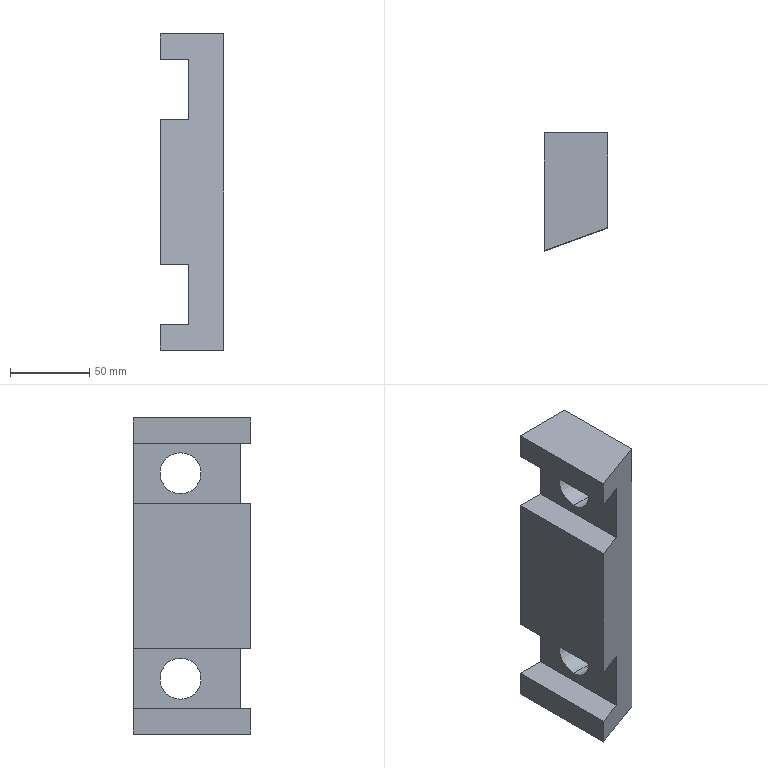Part | SolidWorks | features ICE 2, Extrusion 1, MirrorPattern 1 | 1 solid | 18 faces | box 40 x 74.559 x 200 mm | volume 417359 mm3 | plane 14 | cylinder 4 | commonest cylinder face diameters 26 x4
STEP:
#1=CARTESIAN_POINT('',(40.,44.559,78.));
#2=VERTEX_POINT('',#1);
#3=CARTESIAN_POINT('',(40.,44.559,52.));
#4=VERTEX_POINT('',#3);
#5=CARTESIAN_POINT('',(40.,44.559,65.));
#6=DIRECTION('',(1.,0.,0.));
#7=DIRECTION('',(0.,-1.,0.));
#8=AXIS2_PLACEMENT_3D('',#5,#6,#7);
#9=CIRCLE('',#8,13.);
#10=EDGE_CURVE('',#2,#4,#9,.T.);
#11=ORIENTED_EDGE('',*,*,#10,.T.);
#12=CARTESIAN_POINT('',(18.,44.559,52.));
#13=VERTEX_POINT('',#12);
#14=CARTESIAN_POINT('',(60.,44.559,52.));
#15=DIRECTION('',(-1.,0.,0.));
#16=VECTOR('',#15,1000.);
#17=LINE('',#14,#16);
#18=EDGE_CURVE('',#4,#13,#17,.T.);
#19=ORIENTED_EDGE('',*,*,#18,.T.);
#20=CARTESIAN_POINT('',(18.,44.559,78.));
#21=VERTEX_POINT('',#20);
#22=CARTESIAN_POINT('',(18.,44.559,65.));
#23=DIRECTION('',(1.,0.,0.));
#24=DIRECTION('',(0.,0.,1.));
#25=AXIS2_PLACEMENT_3D('',#22,#23,#24);
#26=CIRCLE('',#25,13.);
#27=EDGE_CURVE('',#21,#13,#26,.T.);
#28=ORIENTED_EDGE('',*,*,#27,.F.);
#29=CARTESIAN_POINT('',(60.,44.559,78.));
#30=DIRECTION('',(-1.,0.,0.));
#31=VECTOR('',#30,1000.);
#32=LINE('',#29,#31);
#33=EDGE_CURVE('',#2,#21,#32,.T.);
#34=ORIENTED_EDGE('',*,*,#33,.F.);
#35=EDGE_LOOP('',(#11,#19,#28,#34));
#36=FACE_OUTER_BOUND('',#35,.T.);
#37=CARTESIAN_POINT('',(60.,44.559,65.));
#38=DIRECTION('',(-1.,0.,0.));
#39=DIRECTION('',(0.,0.,1.));
#40=AXIS2_PLACEMENT_3D('',#37,#38,#39);
#41=CYLINDRICAL_SURFACE('',#40,13.);
#42=ADVANCED_FACE('',(#36),#41,.F.);
#43=CARTESIAN_POINT('',(40.,44.559,-52.));
#44=VERTEX_POINT('',#43);
#45=CARTESIAN_POINT('',(40.,44.559,-78.));
#46=VERTEX_POINT('',#45);
#47=CARTESIAN_POINT('',(40.,44.559,-65.));
#48=DIRECTION('',(1.,0.,0.));
#49=DIRECTION('',(0.,-1.,0.));
#50=AXIS2_PLACEMENT_3D('',#47,#48,#49);
#51=CIRCLE('',#50,13.);
#52=EDGE_CURVE('',#44,#46,#51,.T.);
#53=ORIENTED_EDGE('',*,*,#52,.T.);
#54=CARTESIAN_POINT('',(18.,44.559,-78.));
#55=VERTEX_POINT('',#54);
#56=CARTESIAN_POINT('',(60.,44.559,-78.));
#57=DIRECTION('',(-1.,0.,0.));
#58=VECTOR('',#57,1000.);
#59=LINE('',#56,#58);
#60=EDGE_CURVE('',#46,#55,#59,.T.);
#61=ORIENTED_EDGE('',*,*,#60,.T.);
#62=CARTESIAN_POINT('',(18.,44.559,-52.));
#63=VERTEX_POINT('',#62);
#64=CARTESIAN_POINT('',(18.,44.559,-65.));
#65=DIRECTION('',(1.,0.,0.));
#66=DIRECTION('',(0.,0.,1.));
#67=AXIS2_PLACEMENT_3D('',#64,#65,#66);
#68=CIRCLE('',#67,13.);
#69=EDGE_CURVE('',#63,#55,#68,.T.);
#70=ORIENTED_EDGE('',*,*,#69,.F.);
#71=CARTESIAN_POINT('',(60.,44.559,-52.));
#72=DIRECTION('',(-1.,0.,0.));
#73=VECTOR('',#72,1000.);
#74=LINE('',#71,#73);
#75=EDGE_CURVE('',#44,#63,#74,.T.);
#76=ORIENTED_EDGE('',*,*,#75,.F.);
#77=EDGE_LOOP('',(#53,#61,#70,#76));
#78=FACE_OUTER_BOUND('',#77,.T.);
#79=CARTESIAN_POINT('',(60.,44.559,-65.));
#80=DIRECTION('',(-1.,0.,0.));
#81=DIRECTION('',(0.,0.,1.));
#82=AXIS2_PLACEMENT_3D('',#79,#80,#81);
#83=CYLINDRICAL_SURFACE('',#82,13.);
#84=ADVANCED_FACE('',(#78),#83,.F.);
#85=CARTESIAN_POINT('',(18.,6.551,84.));
#86=VERTEX_POINT('',#85);
#87=CARTESIAN_POINT('',(0.,0.,84.));
#88=VERTEX_POINT('',#87);
#89=CARTESIAN_POINT('',(40.,14.559,84.));
#90=DIRECTION('',(-0.9397,-0.342,0.));
#91=VECTOR('',#90,1000.);
#92=LINE('',#89,#91);
#93=EDGE_CURVE('',#86,#88,#92,.T.);
#94=ORIENTED_EDGE('',*,*,#93,.F.);
#95=CARTESIAN_POINT('',(18.,6.551,46.));
#96=VERTEX_POINT('',#95);
#97=CARTESIAN_POINT('',(18.,6.551,100.));
#98=DIRECTION('',(0.,0.,1.));
#99=VECTOR('',#98,1000.);
#100=LINE('',#97,#99);
#101=EDGE_CURVE('',#96,#86,#100,.T.);
#102=ORIENTED_EDGE('',*,*,#101,.F.);
#103=CARTESIAN_POINT('',(0.,0.,46.));
#104=VERTEX_POINT('',#103);
#105=CARTESIAN_POINT('',(40.,14.559,46.));
#106=DIRECTION('',(0.9397,0.342,0.));
#107=VECTOR('',#106,1000.);
#108=LINE('',#105,#107);
#109=EDGE_CURVE('',#104,#96,#108,.T.);
#110=ORIENTED_EDGE('',*,*,#109,.F.);
#111=CARTESIAN_POINT('',(0.,0.,-46.));
#112=VERTEX_POINT('',#111);
#113=CARTESIAN_POINT('',(0.,0.,100.));
#114=DIRECTION('',(0.,0.,-1.));
#115=VECTOR('',#114,1000.);
#116=LINE('',#113,#115);
#117=EDGE_CURVE('',#104,#112,#116,.T.);
#118=ORIENTED_EDGE('',*,*,#117,.T.);
#119=CARTESIAN_POINT('',(18.,6.551,-46.));
#120=VERTEX_POINT('',#119);
#121=CARTESIAN_POINT('',(40.,14.559,-46.));
#122=DIRECTION('',(0.9397,0.342,0.));
#123=VECTOR('',#122,1000.);
#124=LINE('',#121,#123);
#125=EDGE_CURVE('',#112,#120,#124,.T.);
#126=ORIENTED_EDGE('',*,*,#125,.T.);
#127=CARTESIAN_POINT('',(18.,6.551,-84.));
#128=VERTEX_POINT('',#127);
#129=CARTESIAN_POINT('',(18.,6.551,100.));
#130=DIRECTION('',(0.,0.,1.));
#131=VECTOR('',#130,1000.);
#132=LINE('',#129,#131);
#133=EDGE_CURVE('',#128,#120,#132,.T.);
#134=ORIENTED_EDGE('',*,*,#133,.F.);
#135=CARTESIAN_POINT('',(0.,0.,-84.));
#136=VERTEX_POINT('',#135);
#137=CARTESIAN_POINT('',(40.,14.559,-84.));
#138=DIRECTION('',(-0.9397,-0.342,0.));
#139=VECTOR('',#138,1000.);
#140=LINE('',#137,#139);
#141=EDGE_CURVE('',#128,#136,#140,.T.);
#142=ORIENTED_EDGE('',*,*,#141,.T.);
#143=CARTESIAN_POINT('',(0.,0.,-100.));
#144=VERTEX_POINT('',#143);
#145=CARTESIAN_POINT('',(0.,0.,100.));
#146=DIRECTION('',(0.,0.,-1.));
#147=VECTOR('',#146,1000.);
#148=LINE('',#145,#147);
#149=EDGE_CURVE('',#136,#144,#148,.T.);
#150=ORIENTED_EDGE('',*,*,#149,.T.);
#151=CARTESIAN_POINT('',(40.,14.559,-100.));
#152=VERTEX_POINT('',#151);
#153=CARTESIAN_POINT('',(40.,14.559,-100.));
#154=DIRECTION('',(0.9397,0.342,0.));
#155=VECTOR('',#154,1000.);
#156=LINE('',#153,#155);
#157=EDGE_CURVE('',#144,#152,#156,.T.);
#158=ORIENTED_EDGE('',*,*,#157,.T.);
#159=CARTESIAN_POINT('',(40.,14.559,100.));
#160=VERTEX_POINT('',#159);
#161=CARTESIAN_POINT('',(40.,14.559,100.));
#162=DIRECTION('',(0.,0.,-1.));
#163=VECTOR('',#162,1000.);
#164=LINE('',#161,#163);
#165=EDGE_CURVE('',#160,#152,#164,.T.);
#166=ORIENTED_EDGE('',*,*,#165,.F.);
#167=CARTESIAN_POINT('',(0.,0.,100.));
#168=VERTEX_POINT('',#167);
#169=CARTESIAN_POINT('',(40.,14.559,100.));
#170=DIRECTION('',(0.9397,0.342,0.));
#171=VECTOR('',#170,1000.);
#172=LINE('',#169,#171);
#173=EDGE_CURVE('',#168,#160,#172,.T.);
#174=ORIENTED_EDGE('',*,*,#173,.F.);
#175=CARTESIAN_POINT('',(0.,0.,100.));
#176=DIRECTION('',(0.,0.,-1.));
#177=VECTOR('',#176,1000.);
#178=LINE('',#175,#177);
#179=EDGE_CURVE('',#168,#88,#178,.T.);
#180=ORIENTED_EDGE('',*,*,#179,.T.);
#181=EDGE_LOOP('',(#94,#102,#110,#118,#126,#134,#142,#150,#158,#166,#174,#180));
#182=FACE_OUTER_BOUND('',#181,.T.);
#183=CARTESIAN_POINT('',(40.,14.559,100.));
#184=DIRECTION('',(-0.342,0.9397,0.));
#185=DIRECTION('',(-0.9397,-0.342,0.));
#186=AXIS2_PLACEMENT_3D('',#183,#184,#185);
#187=PLANE('',#186);
#188=ADVANCED_FACE('',(#182),#187,.F.);
#189=CARTESIAN_POINT('',(0.,74.559,84.));
#190=VERTEX_POINT('',#189);
#191=CARTESIAN_POINT('',(18.,74.559,84.));
#192=VERTEX_POINT('',#191);
#193=CARTESIAN_POINT('',(0.,74.559,84.));
#194=DIRECTION('',(1.,0.,0.));
#195=VECTOR('',#194,1000.);
#196=LINE('',#193,#195);
#197=EDGE_CURVE('',#190,#192,#196,.T.);
#198=ORIENTED_EDGE('',*,*,#197,.F.);
#199=CARTESIAN_POINT('',(0.,74.559,100.));
#200=VERTEX_POINT('',#199);
#201=CARTESIAN_POINT('',(0.,74.559,100.));
#202=DIRECTION('',(0.,0.,-1.));
#203=VECTOR('',#202,1000.);
#204=LINE('',#201,#203);
#205=EDGE_CURVE('',#200,#190,#204,.T.);
#206=ORIENTED_EDGE('',*,*,#205,.F.);
#207=CARTESIAN_POINT('',(40.,74.559,100.));
#208=VERTEX_POINT('',#207);
#209=CARTESIAN_POINT('',(0.,74.559,100.));
#210=DIRECTION('',(-1.,0.,0.));
#211=VECTOR('',#210,1000.);
#212=LINE('',#209,#211);
#213=EDGE_CURVE('',#208,#200,#212,.T.);
#214=ORIENTED_EDGE('',*,*,#213,.F.);
#215=CARTESIAN_POINT('',(40.,74.559,-100.));
#216=VERTEX_POINT('',#215);
#217=CARTESIAN_POINT('',(40.,74.559,100.));
#218=DIRECTION('',(0.,0.,-1.));
#219=VECTOR('',#218,1000.);
#220=LINE('',#217,#219);
#221=EDGE_CURVE('',#208,#216,#220,.T.);
#222=ORIENTED_EDGE('',*,*,#221,.T.);
#223=CARTESIAN_POINT('',(0.,74.559,-100.));
#224=VERTEX_POINT('',#223);
#225=CARTESIAN_POINT('',(0.,74.559,-100.));
#226=DIRECTION('',(-1.,0.,0.));
#227=VECTOR('',#226,1000.);
#228=LINE('',#225,#227);
#229=EDGE_CURVE('',#216,#224,#228,.T.);
#230=ORIENTED_EDGE('',*,*,#229,.T.);
#231=CARTESIAN_POINT('',(0.,74.559,-84.));
#232=VERTEX_POINT('',#231);
#233=CARTESIAN_POINT('',(0.,74.559,100.));
#234=DIRECTION('',(0.,0.,-1.));
#235=VECTOR('',#234,1000.);
#236=LINE('',#233,#235);
#237=EDGE_CURVE('',#232,#224,#236,.T.);
#238=ORIENTED_EDGE('',*,*,#237,.F.);
#239=CARTESIAN_POINT('',(18.,74.559,-84.));
#240=VERTEX_POINT('',#239);
#241=CARTESIAN_POINT('',(0.,74.559,-84.));
#242=DIRECTION('',(1.,0.,0.));
#243=VECTOR('',#242,1000.);
#244=LINE('',#241,#243);
#245=EDGE_CURVE('',#232,#240,#244,.T.);
#246=ORIENTED_EDGE('',*,*,#245,.T.);
#247=CARTESIAN_POINT('',(18.,74.559,-46.));
#248=VERTEX_POINT('',#247);
#249=CARTESIAN_POINT('',(18.,74.559,100.));
#250=DIRECTION('',(0.,0.,-1.));
#251=VECTOR('',#250,1000.);
#252=LINE('',#249,#251);
#253=EDGE_CURVE('',#248,#240,#252,.T.);
#254=ORIENTED_EDGE('',*,*,#253,.F.);
#255=CARTESIAN_POINT('',(0.,74.559,-46.));
#256=VERTEX_POINT('',#255);
#257=CARTESIAN_POINT('',(0.,74.559,-46.));
#258=DIRECTION('',(-1.,0.,0.));
#259=VECTOR('',#258,1000.);
#260=LINE('',#257,#259);
#261=EDGE_CURVE('',#248,#256,#260,.T.);
#262=ORIENTED_EDGE('',*,*,#261,.T.);
#263=CARTESIAN_POINT('',(0.,74.559,46.));
#264=VERTEX_POINT('',#263);
#265=CARTESIAN_POINT('',(0.,74.559,100.));
#266=DIRECTION('',(0.,0.,-1.));
#267=VECTOR('',#266,1000.);
#268=LINE('',#265,#267);
#269=EDGE_CURVE('',#264,#256,#268,.T.);
#270=ORIENTED_EDGE('',*,*,#269,.F.);
#271=CARTESIAN_POINT('',(18.,74.559,46.));
#272=VERTEX_POINT('',#271);
#273=CARTESIAN_POINT('',(0.,74.559,46.));
#274=DIRECTION('',(-1.,0.,0.));
#275=VECTOR('',#274,1000.);
#276=LINE('',#273,#275);
#277=EDGE_CURVE('',#272,#264,#276,.T.);
#278=ORIENTED_EDGE('',*,*,#277,.F.);
#279=CARTESIAN_POINT('',(18.,74.559,100.));
#280=DIRECTION('',(0.,0.,-1.));
#281=VECTOR('',#280,1000.);
#282=LINE('',#279,#281);
#283=EDGE_CURVE('',#192,#272,#282,.T.);
#284=ORIENTED_EDGE('',*,*,#283,.F.);
#285=EDGE_LOOP('',(#198,#206,#214,#222,#230,#238,#246,#254,#262,#270,#278,#284));
#286=FACE_OUTER_BOUND('',#285,.T.);
#287=CARTESIAN_POINT('',(0.,74.559,100.));
#288=DIRECTION('',(0.,-1.,0.));
#289=DIRECTION('',(0.,0.,-1.));
#290=AXIS2_PLACEMENT_3D('',#287,#288,#289);
#291=PLANE('',#290);
#292=ADVANCED_FACE('',(#286),#291,.F.);
#293=CARTESIAN_POINT('',(0.,0.,84.));
#294=DIRECTION('',(0.,1.,0.));
#295=VECTOR('',#294,1000.);
#296=LINE('',#293,#295);
#297=EDGE_CURVE('',#88,#190,#296,.T.);
#298=ORIENTED_EDGE('',*,*,#297,.F.);
#299=ORIENTED_EDGE('',*,*,#179,.F.);
#300=CARTESIAN_POINT('',(0.,0.,100.));
#301=DIRECTION('',(0.,-1.,0.));
#302=VECTOR('',#301,1000.);
#303=LINE('',#300,#302);
#304=EDGE_CURVE('',#200,#168,#303,.T.);
#305=ORIENTED_EDGE('',*,*,#304,.F.);
#306=ORIENTED_EDGE('',*,*,#205,.T.);
#307=EDGE_LOOP('',(#298,#299,#305,#306));
#308=FACE_OUTER_BOUND('',#307,.T.);
#309=CARTESIAN_POINT('',(0.,0.,100.));
#310=DIRECTION('',(1.,0.,0.));
#311=DIRECTION('',(0.,0.,-1.));
#312=AXIS2_PLACEMENT_3D('',#309,#310,#311);
#313=PLANE('',#312);
#314=ADVANCED_FACE('',(#308),#313,.F.);
#315=CARTESIAN_POINT('',(0.,0.,46.));
#316=DIRECTION('',(0.,-1.,0.));
#317=VECTOR('',#316,1000.);
#318=LINE('',#315,#317);
#319=EDGE_CURVE('',#264,#104,#318,.T.);
#320=ORIENTED_EDGE('',*,*,#319,.F.);
#321=ORIENTED_EDGE('',*,*,#269,.T.);
#322=CARTESIAN_POINT('',(0.,0.,-46.));
#323=DIRECTION('',(0.,-1.,0.));
#324=VECTOR('',#323,1000.);
#325=LINE('',#322,#324);
#326=EDGE_CURVE('',#256,#112,#325,.T.);
#327=ORIENTED_EDGE('',*,*,#326,.T.);
#328=ORIENTED_EDGE('',*,*,#117,.F.);
#329=EDGE_LOOP('',(#320,#321,#327,#328));
#330=FACE_OUTER_BOUND('',#329,.T.);
#331=CARTESIAN_POINT('',(0.,0.,100.));
#332=DIRECTION('',(1.,0.,0.));
#333=DIRECTION('',(0.,0.,-1.));
#334=AXIS2_PLACEMENT_3D('',#331,#332,#333);
#335=PLANE('',#334);
#336=ADVANCED_FACE('',(#330),#335,.F.);
#337=ORIENTED_EDGE('',*,*,#149,.F.);
#338=CARTESIAN_POINT('',(0.,0.,-84.));
#339=DIRECTION('',(0.,1.,0.));
#340=VECTOR('',#339,1000.);
#341=LINE('',#338,#340);
#342=EDGE_CURVE('',#136,#232,#341,.T.);
#343=ORIENTED_EDGE('',*,*,#342,.T.);
#344=ORIENTED_EDGE('',*,*,#237,.T.);
#345=CARTESIAN_POINT('',(0.,0.,-100.));
#346=DIRECTION('',(0.,-1.,0.));
#347=VECTOR('',#346,1000.);
#348=LINE('',#345,#347);
#349=EDGE_CURVE('',#224,#144,#348,.T.);
#350=ORIENTED_EDGE('',*,*,#349,.T.);
#351=EDGE_LOOP('',(#337,#343,#344,#350));
#352=FACE_OUTER_BOUND('',#351,.T.);
#353=CARTESIAN_POINT('',(0.,0.,100.));
#354=DIRECTION('',(1.,0.,0.));
#355=DIRECTION('',(0.,0.,-1.));
#356=AXIS2_PLACEMENT_3D('',#353,#354,#355);
#357=PLANE('',#356);
#358=ADVANCED_FACE('',(#352),#357,.F.);
#359=ORIENTED_EDGE('',*,*,#10,.F.);
#360=CARTESIAN_POINT('',(40.,44.559,65.));
#361=DIRECTION('',(1.,0.,0.));
#362=DIRECTION('',(0.,-1.,0.));
#363=AXIS2_PLACEMENT_3D('',#360,#361,#362);
#364=CIRCLE('',#363,13.);
#365=EDGE_CURVE('',#4,#2,#364,.T.);
#366=ORIENTED_EDGE('',*,*,#365,.F.);
#367=EDGE_LOOP('',(#359,#366));
#368=FACE_BOUND('',#367,.T.);
#369=ORIENTED_EDGE('',*,*,#52,.F.);
#370=CARTESIAN_POINT('',(40.,44.559,-65.));
#371=DIRECTION('',(1.,0.,0.));
#372=DIRECTION('',(0.,-1.,0.));
#373=AXIS2_PLACEMENT_3D('',#370,#371,#372);
#374=CIRCLE('',#373,13.);
#375=EDGE_CURVE('',#46,#44,#374,.T.);
#376=ORIENTED_EDGE('',*,*,#375,.F.);
#377=EDGE_LOOP('',(#369,#376));
#378=FACE_BOUND('',#377,.T.);
#379=CARTESIAN_POINT('',(40.,74.559,-100.));
#380=DIRECTION('',(0.,1.,0.));
#381=VECTOR('',#380,1000.);
#382=LINE('',#379,#381);
#383=EDGE_CURVE('',#152,#216,#382,.T.);
#384=ORIENTED_EDGE('',*,*,#383,.T.);
#385=ORIENTED_EDGE('',*,*,#221,.F.);
#386=CARTESIAN_POINT('',(40.,74.559,100.));
#387=DIRECTION('',(0.,1.,0.));
#388=VECTOR('',#387,1000.);
#389=LINE('',#386,#388);
#390=EDGE_CURVE('',#160,#208,#389,.T.);
#391=ORIENTED_EDGE('',*,*,#390,.F.);
#392=ORIENTED_EDGE('',*,*,#165,.T.);
#393=EDGE_LOOP('',(#384,#385,#391,#392));
#394=FACE_OUTER_BOUND('',#393,.T.);
#395=CARTESIAN_POINT('',(40.,74.559,100.));
#396=DIRECTION('',(-1.,0.,0.));
#397=DIRECTION('',(0.,-1.,0.));
#398=AXIS2_PLACEMENT_3D('',#395,#396,#397);
#399=PLANE('',#398);
#400=ADVANCED_FACE('',(#368,#378,#394),#399,.F.);
#401=ORIENTED_EDGE('',*,*,#173,.T.);
#402=ORIENTED_EDGE('',*,*,#390,.T.);
#403=ORIENTED_EDGE('',*,*,#213,.T.);
#404=ORIENTED_EDGE('',*,*,#304,.T.);
#405=EDGE_LOOP('',(#401,#402,#403,#404));
#406=FACE_OUTER_BOUND('',#405,.T.);
#407=CARTESIAN_POINT('',(0.,0.,100.));
#408=DIRECTION('',(0.,0.,-1.));
#409=DIRECTION('',(-1.,0.,0.));
#410=AXIS2_PLACEMENT_3D('',#407,#408,#409);
#411=PLANE('',#410);
#412=ADVANCED_FACE('',(#406),#411,.F.);
#413=ORIENTED_EDGE('',*,*,#157,.F.);
#414=ORIENTED_EDGE('',*,*,#349,.F.);
#415=ORIENTED_EDGE('',*,*,#229,.F.);
#416=ORIENTED_EDGE('',*,*,#383,.F.);
#417=EDGE_LOOP('',(#413,#414,#415,#416));
#418=FACE_OUTER_BOUND('',#417,.T.);
#419=CARTESIAN_POINT('',(0.,0.,-100.));
#420=DIRECTION('',(0.,0.,-1.));
#421=DIRECTION('',(-1.,0.,0.));
#422=AXIS2_PLACEMENT_3D('',#419,#420,#421);
#423=PLANE('',#422);
#424=ADVANCED_FACE('',(#418),#423,.T.);
#425=ORIENTED_EDGE('',*,*,#69,.T.);
#426=CARTESIAN_POINT('',(18.,44.559,-65.));
#427=DIRECTION('',(1.,0.,0.));
#428=DIRECTION('',(0.,0.,1.));
#429=AXIS2_PLACEMENT_3D('',#426,#427,#428);
#430=CIRCLE('',#429,13.);
#431=EDGE_CURVE('',#55,#63,#430,.T.);
#432=ORIENTED_EDGE('',*,*,#431,.T.);
#433=EDGE_LOOP('',(#425,#432));
#434=FACE_BOUND('',#433,.T.);
#435=ORIENTED_EDGE('',*,*,#133,.T.);
#436=CARTESIAN_POINT('',(18.,-16.656,-46.));
#437=DIRECTION('',(0.,1.,0.));
#438=VECTOR('',#437,1000.);
#439=LINE('',#436,#438);
#440=EDGE_CURVE('',#120,#248,#439,.T.);
#441=ORIENTED_EDGE('',*,*,#440,.T.);
#442=ORIENTED_EDGE('',*,*,#253,.T.);
#443=CARTESIAN_POINT('',(18.,-16.656,-84.));
#444=DIRECTION('',(0.,-1.,0.));
#445=VECTOR('',#444,1000.);
#446=LINE('',#443,#445);
#447=EDGE_CURVE('',#240,#128,#446,.T.);
#448=ORIENTED_EDGE('',*,*,#447,.T.);
#449=EDGE_LOOP('',(#435,#441,#442,#448));
#450=FACE_OUTER_BOUND('',#449,.T.);
#451=CARTESIAN_POINT('',(18.,0.,0.));
#452=DIRECTION('',(-1.,0.,0.));
#453=DIRECTION('',(0.,0.,1.));
#454=AXIS2_PLACEMENT_3D('',#451,#452,#453);
#455=PLANE('',#454);
#456=ADVANCED_FACE('',(#434,#450),#455,.T.);
#457=ORIENTED_EDGE('',*,*,#447,.F.);
#458=ORIENTED_EDGE('',*,*,#245,.F.);
#459=ORIENTED_EDGE('',*,*,#342,.F.);
#460=ORIENTED_EDGE('',*,*,#141,.F.);
#461=EDGE_LOOP('',(#457,#458,#459,#460));
#462=FACE_OUTER_BOUND('',#461,.T.);
#463=CARTESIAN_POINT('',(18.,-16.656,-84.));
#464=DIRECTION('',(0.,0.,-1.));
#465=DIRECTION('',(-1.,0.,0.));
#466=AXIS2_PLACEMENT_3D('',#463,#464,#465);
#467=PLANE('',#466);
#468=ADVANCED_FACE('',(#462),#467,.F.);
#469=ORIENTED_EDGE('',*,*,#326,.F.);
#470=ORIENTED_EDGE('',*,*,#261,.F.);
#471=ORIENTED_EDGE('',*,*,#440,.F.);
#472=ORIENTED_EDGE('',*,*,#125,.F.);
#473=EDGE_LOOP('',(#469,#470,#471,#472));
#474=FACE_OUTER_BOUND('',#473,.T.);
#475=CARTESIAN_POINT('',(18.,-16.656,-46.));
#476=DIRECTION('',(0.,0.,1.));
#477=DIRECTION('',(1.,0.,0.));
#478=AXIS2_PLACEMENT_3D('',#475,#476,#477);
#479=PLANE('',#478);
#480=ADVANCED_FACE('',(#474),#479,.F.);
#481=ORIENTED_EDGE('',*,*,#27,.T.);
#482=CARTESIAN_POINT('',(18.,44.559,65.));
#483=DIRECTION('',(1.,0.,0.));
#484=DIRECTION('',(0.,0.,1.));
#485=AXIS2_PLACEMENT_3D('',#482,#483,#484);
#486=CIRCLE('',#485,13.);
#487=EDGE_CURVE('',#13,#21,#486,.T.);
#488=ORIENTED_EDGE('',*,*,#487,.T.);
#489=EDGE_LOOP('',(#481,#488));
#490=FACE_BOUND('',#489,.T.);
#491=ORIENTED_EDGE('',*,*,#101,.T.);
#492=CARTESIAN_POINT('',(18.,-16.656,84.));
#493=DIRECTION('',(0.,-1.,0.));
#494=VECTOR('',#493,1000.);
#495=LINE('',#492,#494);
#496=EDGE_CURVE('',#192,#86,#495,.T.);
#497=ORIENTED_EDGE('',*,*,#496,.F.);
#498=ORIENTED_EDGE('',*,*,#283,.T.);
#499=CARTESIAN_POINT('',(18.,-16.656,46.));
#500=DIRECTION('',(0.,1.,0.));
#501=VECTOR('',#500,1000.);
#502=LINE('',#499,#501);
#503=EDGE_CURVE('',#96,#272,#502,.T.);
#504=ORIENTED_EDGE('',*,*,#503,.F.);
#505=EDGE_LOOP('',(#491,#497,#498,#504));
#506=FACE_OUTER_BOUND('',#505,.T.);
#507=CARTESIAN_POINT('',(18.,0.,0.));
#508=DIRECTION('',(-1.,0.,0.));
#509=DIRECTION('',(0.,0.,-1.));
#510=AXIS2_PLACEMENT_3D('',#507,#508,#509);
#511=PLANE('',#510);
#512=ADVANCED_FACE('',(#490,#506),#511,.T.);
#513=ORIENTED_EDGE('',*,*,#93,.T.);
#514=ORIENTED_EDGE('',*,*,#297,.T.);
#515=ORIENTED_EDGE('',*,*,#197,.T.);
#516=ORIENTED_EDGE('',*,*,#496,.T.);
#517=EDGE_LOOP('',(#513,#514,#515,#516));
#518=FACE_OUTER_BOUND('',#517,.T.);
#519=CARTESIAN_POINT('',(18.,-16.656,84.));
#520=DIRECTION('',(0.,0.,-1.));
#521=DIRECTION('',(-1.,0.,0.));
#522=AXIS2_PLACEMENT_3D('',#519,#520,#521);
#523=PLANE('',#522);
#524=ADVANCED_FACE('',(#518),#523,.T.);
#525=ORIENTED_EDGE('',*,*,#109,.T.);
#526=ORIENTED_EDGE('',*,*,#503,.T.);
#527=ORIENTED_EDGE('',*,*,#277,.T.);
#528=ORIENTED_EDGE('',*,*,#319,.T.);
#529=EDGE_LOOP('',(#525,#526,#527,#528));
#530=FACE_OUTER_BOUND('',#529,.T.);
#531=CARTESIAN_POINT('',(18.,-16.656,46.));
#532=DIRECTION('',(0.,0.,1.));
#533=DIRECTION('',(1.,0.,0.));
#534=AXIS2_PLACEMENT_3D('',#531,#532,#533);
#535=PLANE('',#534);
#536=ADVANCED_FACE('',(#530),#535,.T.);
#537=ORIENTED_EDGE('',*,*,#60,.F.);
#538=ORIENTED_EDGE('',*,*,#375,.T.);
#539=ORIENTED_EDGE('',*,*,#75,.T.);
#540=ORIENTED_EDGE('',*,*,#431,.F.);
#541=EDGE_LOOP('',(#537,#538,#539,#540));
#542=FACE_OUTER_BOUND('',#541,.T.);
#543=CARTESIAN_POINT('',(60.,44.559,-65.));
#544=DIRECTION('',(-1.,0.,0.));
#545=DIRECTION('',(0.,0.,1.));
#546=AXIS2_PLACEMENT_3D('',#543,#544,#545);
#547=CYLINDRICAL_SURFACE('',#546,13.);
#548=ADVANCED_FACE('',(#542),#547,.F.);
#549=ORIENTED_EDGE('',*,*,#18,.F.);
#550=ORIENTED_EDGE('',*,*,#365,.T.);
#551=ORIENTED_EDGE('',*,*,#33,.T.);
#552=ORIENTED_EDGE('',*,*,#487,.F.);
#553=EDGE_LOOP('',(#549,#550,#551,#552));
#554=FACE_OUTER_BOUND('',#553,.T.);
#555=CARTESIAN_POINT('',(60.,44.559,65.));
#556=DIRECTION('',(-1.,0.,0.));
#557=DIRECTION('',(0.,0.,1.));
#558=AXIS2_PLACEMENT_3D('',#555,#556,#557);
#559=CYLINDRICAL_SURFACE('',#558,13.);
#560=ADVANCED_FACE('',(#554),#559,.F.);
#561=CLOSED_SHELL('',(#42,#84,#188,#292,#314,#336,#358,#400,#412,#424,#456,#468,#480,#512,#524,#536,#548,#560));
#562=MANIFOLD_SOLID_BREP('',#561);
#563=CARTESIAN_POINT('',(0.,0.,0.));
#564=DIRECTION('',(0.,0.,1.));
#565=DIRECTION('',(1.,0.,0.));
#566=AXIS2_PLACEMENT_3D('',#563,#564,#565);
#567=(LENGTH_UNIT()NAMED_UNIT(*)SI_UNIT(.MILLI.,.METRE.));
#568=UNCERTAINTY_MEASURE_WITH_UNIT(LENGTH_MEASURE(0.00001),#567,'','');
#569=(NAMED_UNIT(*)PLANE_ANGLE_UNIT()SI_UNIT($,.RADIAN.));
#570=(NAMED_UNIT(*)SI_UNIT($,.STERADIAN.)SOLID_ANGLE_UNIT());
#571=(GEOMETRIC_REPRESENTATION_CONTEXT(3)GLOBAL_UNCERTAINTY_ASSIGNED_CONTEXT((#568))GLOBAL_UNIT_ASSIGNED_CONTEXT((#567,#569,#570))REPRESENTATION_CONTEXT('',''));
#572=ADVANCED_BREP_SHAPE_REPRESENTATION('',(#562,#566),#571);